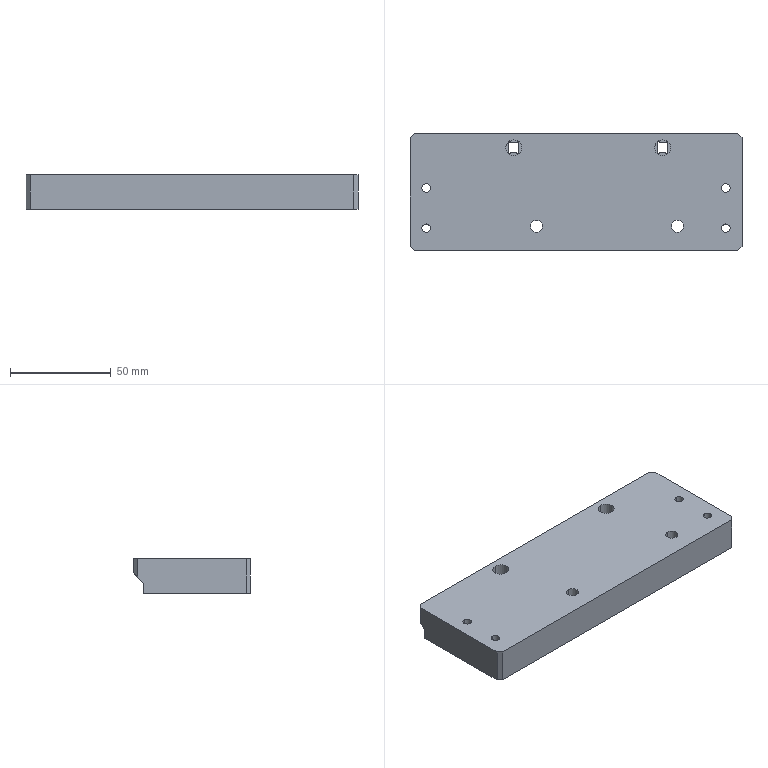NC program | NX | posted with a generic post | part box 165 x 58 x 17 mm
Lines 3545 to 3780 of 3780:
(PLANAR_MILL_COPY , TOOL : D6A45)
N7016 T01 M6
N7018 G54
N7020 G17 G0 G90 X77.63 Y-14.65 S9500 M3
N7022 G43 Z30. H1
N7024 Z0.5
N7026 G94 G1 Z-1. F1250.
N7028 X78.33 Y-14.246
N7030 G3 X78.83 Y-13.38 R1.
N7032 G1 Y-8.735
N7034 X78.843 Y-8.67
N7036 X78.795 Y-8.622
N7038 X78.73 Y-8.635
N7040 X69.73
N7042 X69.665 Y-8.622
N7044 X69.617 Y-8.67
N7046 X69.63 Y-8.735
N7048 Y-18.025
N7050 X69.617 Y-18.09
N7052 X69.665 Y-18.138
N7054 X69.73 Y-18.125
N7056 X78.73
N7058 X78.795 Y-18.138
N7060 X78.843 Y-18.09
N7062 X78.83 Y-18.025
N7064 Y-13.38
N7066 G3 X78.33 Y-12.514 R1.
N7068 G1 X77.63 Y-12.11
N7070 Z0.5
N7072 G0 Z30.
N7074 X74.37 Y-0.8
N7076 Z0.5
N7078 G1 X74.23 Z0.462
N7080 X73.63 Y-1.13 Z0.279
N7082 X73.3 Y-1.73 Z0.096
N7084 Y-2.27 Z-0.049
N7086 X73.63 Y-2.87 Z-0.233
N7088 X74.23 Y-3.2 Z-0.416
N7090 X74.77 Z-0.561
N7092 X75.37 Y-2.87 Z-0.744
N7094 X75.7 Y-2.27 Z-0.928
N7096 Y-2. Z-1.
N7098 G3 X74.5 Y-0.8 R1.2
N7100 X75.7 Y-2. R-1.2
N7102 X75.2 Y-1.134 R1.
N7104 G1 Z0.5
N7106 G0 Z30.
N7108 X74.37 Y19.2
N7110 Z0.5
N7112 G1 X74.23 Z0.462
N7114 X73.63 Y18.87 Z0.279
N7116 X73.3 Y18.27 Z0.096
N7118 Y17.73 Z-0.049
N7120 X73.63 Y17.13 Z-0.233
N7122 X74.23 Y16.8 Z-0.416
N7124 X74.77 Z-0.561
N7126 X75.37 Y17.13 Z-0.744
N7128 X75.7 Y17.73 Z-0.928
N7130 Y18. Z-1.
N7132 G3 X74.5 Y19.2 R1.2
N7134 X75.7 Y18. R-1.2
N7136 X75.2 Y18.866 R1.
N7138 G1 Z0.5
N7140 G0 Z30.
N7142 X50.808 Y17.791
N7144 Z0.5
N7146 G1 Z-1.
N7148 X51.246 Y18.6
N7150 G3 X50.38 Y19.1 R1.
N7152 X48.28 Y17. R2.1
N7154 X50.38 Y19.1 R-2.1
N7156 X49.514 Y18.6 R1.
N7158 G1 X49.952 Y17.791
N7160 Z0.5
N7162 G0 Z30.
N7164 X34.804 Y-8.685
N7166 Z0.5
N7168 G1 Z-1.
N7170 X33.865 Y-8.272
N7172 G3 X32.871 Y-8.382 R1.
N7174 X39.926 Y-18.928 R6.35
N7176 G2 X40.511 Y-18.785 R1.
N7178 X40.823 Y-18.269 R1.
N7180 G3 X32.871 Y-8.382 R6.35
N7182 X32.469 Y-9.298 R1.
N7184 G1 X32.582 Y-10.317
N7186 Z0.5
N7188 G0 Z30.
N7190 X-1.04 Y-16.925
N7192 Z0.5
N7194 G1 Z-1.
N7196 X-0.636 Y-17.625
N7198 G3 X0.23 Y-18.125 R1.
N7200 G1 X4.73
N7202 X4.795 Y-18.138
N7204 X4.843 Y-18.09
N7206 X4.83 Y-18.025
N7208 Y-8.735
N7210 X4.843 Y-8.67
N7212 X4.795 Y-8.622
N7214 X4.73 Y-8.635
N7216 X-4.27
N7218 X-4.335 Y-8.622
N7220 X-4.383 Y-8.67
N7222 X-4.37 Y-8.735
N7224 Y-18.025
N7226 X-4.383 Y-18.09
N7228 X-4.335 Y-18.138
N7230 X-4.27 Y-18.125
N7232 X0.23
N7234 G3 X1.096 Y-17.625 R1.
N7236 G1 X1.5 Y-16.925
N7238 Z0.5
N7240 G0 Z30.
N7242 X-19.192 Y17.791
N7244 Z0.5
N7246 G1 Z-1.
N7248 X-18.754 Y18.6
N7250 G3 X-19.62 Y19.1 R1.
N7252 X-21.72 Y17. R2.1
N7254 X-19.62 Y19.1 R-2.1
N7256 X-20.486 Y18.6 R1.
N7258 G1 X-20.048 Y17.791
N7260 Z0.5
N7262 G0 Z30.
N7264 X-39.196 Y-8.685
N7266 Z0.5
N7268 G1 Z-1.
N7270 X-40.135 Y-8.272
N7272 G3 X-41.129 Y-8.382 R1.
N7274 X-34.074 Y-18.928 R6.35
N7276 G2 X-33.489 Y-18.785 R1.
N7278 X-33.177 Y-18.269 R1.
N7280 G3 X-41.129 Y-8.382 R6.35
N7282 X-41.531 Y-9.298 R1.
N7284 G1 X-41.418 Y-10.317
N7286 Z0.5
N7288 G0 Z30.
N7290 X-74.37 Y-3.2
N7292 Z0.5
N7294 G1 X-74.23 Z0.462
N7296 X-73.63 Y-2.87 Z0.279
N7298 X-73.3 Y-2.27 Z0.096
N7300 Y-1.73 Z-0.049
N7302 X-73.63 Y-1.13 Z-0.233
N7304 X-74.23 Y-0.8 Z-0.416
N7306 X-74.77 Z-0.561
N7308 X-75.37 Y-1.13 Z-0.744
N7310 X-75.7 Y-1.73 Z-0.928
N7312 Y-2. Z-1.
N7314 G3 X-74.5 Y-3.2 R1.2
N7316 X-75.7 Y-2. R-1.2
N7318 X-75.2 Y-2.866 R1.
N7320 G1 Z0.5
N7322 G0 Z30.
N7324 X-74.37 Y16.8
N7326 Z0.5
N7328 G1 X-74.23 Z0.462
N7330 X-73.63 Y17.13 Z0.279
N7332 X-73.3 Y17.73 Z0.096
N7334 Y18.27 Z-0.049
N7336 X-73.63 Y18.87 Z-0.233
N7338 X-74.23 Y19.2 Z-0.416
N7340 X-74.77 Z-0.561
N7342 X-75.37 Y18.87 Z-0.744
N7344 X-75.7 Y18.27 Z-0.928
N7346 Y18. Z-1.
N7348 G3 X-74.5 Y16.8 R1.2
N7350 X-75.7 Y18. R-1.2
N7352 X-75.2 Y17.134 R1.
N7354 G1 Z0.5
N7356 G0 Z30.
(PLANAR_MILL_COPY_COPY , TOOL : D6A45)
N7358 X-84.6 Y-25.27
N7360 Z0.5
N7362 G1 Z-1.
N7364 X-83.9 Y-24.866
N7366 G3 X-83.4 Y-24. R1.
N7368 G1 Y26.959
N7370 G2 X-83.107 Y27.666 R1.
N7372 G1 X-81.166 Y29.607
N7374 G2 X-80.459 Y29.9 R1.
N7376 G1 X80.459
N7378 G2 X81.166 Y29.607 R1.
N7380 G1 X83.107 Y27.666
N7382 G2 X83.4 Y26.959 R1.
N7384 G1 Y-24.
N7386 G3 X83.9 Y-24.866 R1.
N7388 G1 X84.6 Y-25.27
N7390 Z0.5
N7392 G0 Z30.
N7394 M5
(刀补11 , TOOL : D4)
N7396 T11 M6
N7398 G54
N7400 G17 G0 G90 X-19.62 Y17. S9500 M3
N7402 G43 Z30. H11
N7404 Z0.5
N7406 G41 G94 G1 X-19.616 Y16.9 F1250. D11
N7408 G3 X-18.67 Y17. R0.478
N7410 X-18.67 Y17. Z-2.5 I-0.95 J0.
N7412 X-18.67 Y17. Z-5.5 I-0.95 J0.
N7414 X-18.67 Y17. Z-8.5 I-0.95 J0.
N7416 X-18.67 Y17. Z-11.5 I-0.95 J0.
N7418 X-18.67 Y17. Z-14.5 I-0.95 J0.
N7420 X-19.145 Y16.177 Z-17. R-0.95
N7422 X-18.797 Y17.475 R0.95
N7424 X-19.145 Y16.177 R-0.95
N7426 X-19.532 Y17.047 R0.478
N7428 G40
N7430 G1 X-19.62 Y17.
N7432 G0 Z30.
N7434 X50.38
N7436 Z0.5
N7438 G41 G1 X50.384 Y16.9
N7440 G3 X51.33 Y17. R0.478
N7442 X51.33 Y17. Z-2.5 I-0.95 J0.
N7444 X51.33 Y17. Z-5.5 I-0.95 J0.
N7446 X51.33 Y17. Z-8.5 I-0.95 J0.
N7448 X51.33 Y17. Z-11.5 I-0.95 J0.
N7450 X51.33 Y17. Z-14.5 I-0.95 J0.
N7452 X50.855 Y16.177 Z-17. R-0.95
N7454 X51.203 Y17.475 R0.95
N7456 X50.855 Y16.177 R-0.95
N7458 X50.468 Y17.047 R0.478
N7460 G40
N7462 G1 X50.38 Y17.
N7464 G0 Z30.
N7466 M5
N7468 M2